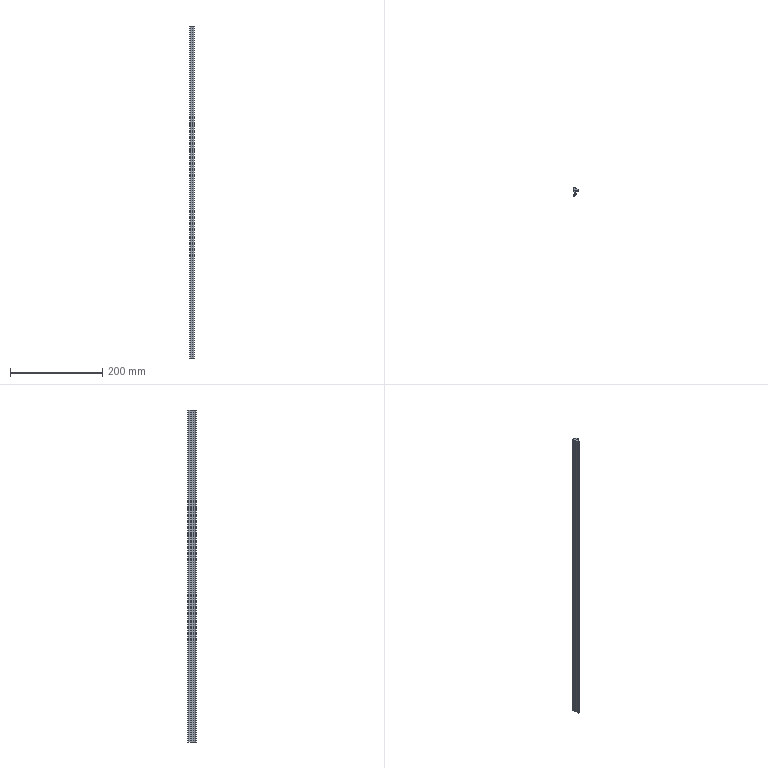Part | STEP file | AMH71封条-408 | 1 solid | 20 faces | box 10.8 x 17.5 x 720 mm | volume 56736 mm3 | cylinder 11 | plane 9 | commonest cylinder face diameters 1.6 x2 14 x2 0.4 x1 0.6 x1 0.8 x1 2.6 x1
STEP:
#1=CARTESIAN_POINT('',(-3.236,-11.055,0.));
#2=VERTEX_POINT('',#1);
#3=CARTESIAN_POINT('',(-4.3,-10.3,0.));
#4=VERTEX_POINT('',#3);
#5=CARTESIAN_POINT('',(-3.5,-10.3,0.));
#6=DIRECTION('',(0.,0.,-1.));
#7=DIRECTION('',(-1.,0.,0.));
#8=AXIS2_PLACEMENT_3D('',#5,#6,#7);
#9=CIRCLE('',#8,0.8);
#10=EDGE_CURVE('',#2,#4,#9,.T.);
#11=ORIENTED_EDGE('',*,*,#10,.T.);
#12=CARTESIAN_POINT('',(-4.3,-10.3,-720.));
#13=VERTEX_POINT('',#12);
#14=CARTESIAN_POINT('',(-4.3,-10.3,-100.));
#15=DIRECTION('',(0.,0.,-1.));
#16=VECTOR('',#15,1000.);
#17=LINE('',#14,#16);
#18=EDGE_CURVE('',#4,#13,#17,.T.);
#19=ORIENTED_EDGE('',*,*,#18,.T.);
#20=CARTESIAN_POINT('',(-3.236,-11.055,-720.));
#21=VERTEX_POINT('',#20);
#22=CARTESIAN_POINT('',(-3.5,-10.3,-720.));
#23=DIRECTION('',(0.,0.,1.));
#24=DIRECTION('',(-1.,0.,0.));
#25=AXIS2_PLACEMENT_3D('',#22,#23,#24);
#26=CIRCLE('',#25,0.8);
#27=EDGE_CURVE('',#13,#21,#26,.T.);
#28=ORIENTED_EDGE('',*,*,#27,.T.);
#29=CARTESIAN_POINT('',(-3.236,-11.055,-100.));
#30=DIRECTION('',(0.,0.,-1.));
#31=VECTOR('',#30,1000.);
#32=LINE('',#29,#31);
#33=EDGE_CURVE('',#2,#21,#32,.T.);
#34=ORIENTED_EDGE('',*,*,#33,.F.);
#35=EDGE_LOOP('',(#11,#19,#28,#34));
#36=FACE_OUTER_BOUND('',#35,.T.);
#37=CARTESIAN_POINT('',(-3.5,-10.3,-100.));
#38=DIRECTION('',(0.,0.,-1.));
#39=DIRECTION('',(-1.,0.,0.));
#40=AXIS2_PLACEMENT_3D('',#37,#38,#39);
#41=CYLINDRICAL_SURFACE('',#40,0.8);
#42=ADVANCED_FACE('',(#36),#41,.T.);
#43=CARTESIAN_POINT('',(1.184,-6.397,-720.));
#44=VERTEX_POINT('',#43);
#45=CARTESIAN_POINT('',(-5.702,-4.29,-720.));
#46=DIRECTION('',(0.,0.,1.));
#47=DIRECTION('',(-1.,0.,0.));
#48=AXIS2_PLACEMENT_3D('',#45,#46,#47);
#49=CIRCLE('',#48,7.201);
#50=EDGE_CURVE('',#21,#44,#49,.T.);
#51=ORIENTED_EDGE('',*,*,#50,.T.);
#52=CARTESIAN_POINT('',(1.184,-6.397,0.));
#53=VERTEX_POINT('',#52);
#54=CARTESIAN_POINT('',(1.184,-6.397,-100.));
#55=DIRECTION('',(0.,0.,1.));
#56=VECTOR('',#55,1000.);
#57=LINE('',#54,#56);
#58=EDGE_CURVE('',#44,#53,#57,.T.);
#59=ORIENTED_EDGE('',*,*,#58,.T.);
#60=CARTESIAN_POINT('',(-5.702,-4.29,0.));
#61=DIRECTION('',(0.,0.,-1.));
#62=DIRECTION('',(-1.,0.,0.));
#63=AXIS2_PLACEMENT_3D('',#60,#61,#62);
#64=CIRCLE('',#63,7.201);
#65=EDGE_CURVE('',#53,#2,#64,.T.);
#66=ORIENTED_EDGE('',*,*,#65,.T.);
#67=ORIENTED_EDGE('',*,*,#33,.T.);
#68=EDGE_LOOP('',(#51,#59,#66,#67));
#69=FACE_OUTER_BOUND('',#68,.T.);
#70=CARTESIAN_POINT('',(-5.702,-4.29,-100.));
#71=DIRECTION('',(0.,0.,-1.));
#72=DIRECTION('',(-1.,0.,0.));
#73=AXIS2_PLACEMENT_3D('',#70,#71,#72);
#74=CYLINDRICAL_SURFACE('',#73,7.201);
#75=ADVANCED_FACE('',(#69),#74,.T.);
#76=CARTESIAN_POINT('',(0.9,-6.,-720.));
#77=VERTEX_POINT('',#76);
#78=CARTESIAN_POINT('',(0.9,-6.3,-720.));
#79=DIRECTION('',(0.,0.,1.));
#80=DIRECTION('',(-1.,0.,0.));
#81=AXIS2_PLACEMENT_3D('',#78,#79,#80);
#82=CIRCLE('',#81,0.3);
#83=EDGE_CURVE('',#44,#77,#82,.T.);
#84=ORIENTED_EDGE('',*,*,#83,.T.);
#85=CARTESIAN_POINT('',(0.9,-6.,0.));
#86=VERTEX_POINT('',#85);
#87=CARTESIAN_POINT('',(0.9,-6.,-100.));
#88=DIRECTION('',(0.,0.,1.));
#89=VECTOR('',#88,1000.);
#90=LINE('',#87,#89);
#91=EDGE_CURVE('',#77,#86,#90,.T.);
#92=ORIENTED_EDGE('',*,*,#91,.T.);
#93=CARTESIAN_POINT('',(0.9,-6.3,0.));
#94=DIRECTION('',(0.,0.,-1.));
#95=DIRECTION('',(-1.,0.,0.));
#96=AXIS2_PLACEMENT_3D('',#93,#94,#95);
#97=CIRCLE('',#96,0.3);
#98=EDGE_CURVE('',#86,#53,#97,.T.);
#99=ORIENTED_EDGE('',*,*,#98,.T.);
#100=ORIENTED_EDGE('',*,*,#58,.F.);
#101=EDGE_LOOP('',(#84,#92,#99,#100));
#102=FACE_OUTER_BOUND('',#101,.T.);
#103=CARTESIAN_POINT('',(0.9,-6.3,-100.));
#104=DIRECTION('',(0.,0.,-1.));
#105=DIRECTION('',(-1.,0.,0.));
#106=AXIS2_PLACEMENT_3D('',#103,#104,#105);
#107=CYLINDRICAL_SURFACE('',#106,0.3);
#108=ADVANCED_FACE('',(#102),#107,.T.);
#109=CARTESIAN_POINT('',(-2.5,-0.5,-720.));
#110=VERTEX_POINT('',#109);
#111=CARTESIAN_POINT('',(-2.5,-6.153,-720.));
#112=VERTEX_POINT('',#111);
#113=CARTESIAN_POINT('',(-2.5,-6.397,-720.));
#114=DIRECTION('',(0.,-1.,0.));
#115=VECTOR('',#114,1000.);
#116=LINE('',#113,#115);
#117=EDGE_CURVE('',#110,#112,#116,.T.);
#118=ORIENTED_EDGE('',*,*,#117,.F.);
#119=CARTESIAN_POINT('',(-4.2,1.695,-720.));
#120=VERTEX_POINT('',#119);
#121=CARTESIAN_POINT('',(-1.701,1.875,-720.));
#122=DIRECTION('',(0.,0.,1.));
#123=DIRECTION('',(-1.,0.,0.));
#124=AXIS2_PLACEMENT_3D('',#121,#122,#123);
#125=CIRCLE('',#124,2.506);
#126=EDGE_CURVE('',#120,#110,#125,.T.);
#127=ORIENTED_EDGE('',*,*,#126,.F.);
#128=CARTESIAN_POINT('',(-4.2,5.1,-720.));
#129=VERTEX_POINT('',#128);
#130=CARTESIAN_POINT('',(-4.2,-6.397,-720.));
#131=DIRECTION('',(0.,-1.,0.));
#132=VECTOR('',#131,1000.);
#133=LINE('',#130,#132);
#134=EDGE_CURVE('',#129,#120,#133,.T.);
#135=ORIENTED_EDGE('',*,*,#134,.F.);
#136=CARTESIAN_POINT('',(-2.892,6.4,-720.));
#137=VERTEX_POINT('',#136);
#138=CARTESIAN_POINT('',(-2.9,5.1,-720.));
#139=DIRECTION('',(0.,0.,1.));
#140=DIRECTION('',(-1.,0.,0.));
#141=AXIS2_PLACEMENT_3D('',#138,#139,#140);
#142=CIRCLE('',#141,1.3);
#143=EDGE_CURVE('',#137,#129,#142,.T.);
#144=ORIENTED_EDGE('',*,*,#143,.F.);
#145=CARTESIAN_POINT('',(0.5,5.5,-720.));
#146=VERTEX_POINT('',#145);
#147=CARTESIAN_POINT('',(-2.934,-0.5999,-720.));
#148=DIRECTION('',(0.,0.,1.));
#149=DIRECTION('',(-1.,0.,0.));
#150=AXIS2_PLACEMENT_3D('',#147,#148,#149);
#151=CIRCLE('',#150,7.);
#152=EDGE_CURVE('',#146,#137,#151,.T.);
#153=ORIENTED_EDGE('',*,*,#152,.F.);
#154=CARTESIAN_POINT('',(5.5,1.7,-720.));
#155=VERTEX_POINT('',#154);
#156=CARTESIAN_POINT('',(5.5,1.7,-720.));
#157=DIRECTION('',(-0.7962,0.6051,0.));
#158=VECTOR('',#157,1000.);
#159=LINE('',#156,#158);
#160=EDGE_CURVE('',#155,#146,#159,.T.);
#161=ORIENTED_EDGE('',*,*,#160,.F.);
#162=CARTESIAN_POINT('',(6.458,-0.2215,-720.));
#163=VERTEX_POINT('',#162);
#164=CARTESIAN_POINT('',(6.458,-0.2215,-720.));
#165=DIRECTION('',(-0.4462,0.8949,0.));
#166=VECTOR('',#165,1000.);
#167=LINE('',#164,#166);
#168=EDGE_CURVE('',#163,#155,#167,.T.);
#169=ORIENTED_EDGE('',*,*,#168,.F.);
#170=CARTESIAN_POINT('',(5.895,-0.7433,-720.));
#171=VERTEX_POINT('',#170);
#172=CARTESIAN_POINT('',(6.1,-0.4,-720.));
#173=DIRECTION('',(0.,0.,1.));
#174=DIRECTION('',(-1.,0.,0.));
#175=AXIS2_PLACEMENT_3D('',#172,#173,#174);
#176=CIRCLE('',#175,0.4);
#177=EDGE_CURVE('',#171,#163,#176,.T.);
#178=ORIENTED_EDGE('',*,*,#177,.F.);
#179=CARTESIAN_POINT('',(3.,0.,-720.));
#180=VERTEX_POINT('',#179);
#181=CARTESIAN_POINT('',(2.746,-6.995,-720.));
#182=DIRECTION('',(0.,0.,-1.));
#183=DIRECTION('',(-1.,0.,0.));
#184=AXIS2_PLACEMENT_3D('',#181,#182,#183);
#185=CIRCLE('',#184,7.);
#186=EDGE_CURVE('',#180,#171,#185,.T.);
#187=ORIENTED_EDGE('',*,*,#186,.F.);
#188=CARTESIAN_POINT('',(0.,0.,-720.));
#189=VERTEX_POINT('',#188);
#190=CARTESIAN_POINT('',(-6.814,0.,-720.));
#191=DIRECTION('',(1.,0.,0.));
#192=VECTOR('',#191,1000.);
#193=LINE('',#190,#192);
#194=EDGE_CURVE('',#189,#180,#193,.T.);
#195=ORIENTED_EDGE('',*,*,#194,.F.);
#196=CARTESIAN_POINT('',(0.,-5.8,-720.));
#197=VERTEX_POINT('',#196);
#198=CARTESIAN_POINT('',(0.,-6.397,-720.));
#199=DIRECTION('',(0.,1.,0.));
#200=VECTOR('',#199,1000.);
#201=LINE('',#198,#200);
#202=EDGE_CURVE('',#197,#189,#201,.T.);
#203=ORIENTED_EDGE('',*,*,#202,.F.);
#204=CARTESIAN_POINT('',(0.2,-6.,-720.));
#205=VERTEX_POINT('',#204);
#206=CARTESIAN_POINT('',(0.2,-5.8,-720.));
#207=DIRECTION('',(0.,0.,1.));
#208=DIRECTION('',(-1.,0.,0.));
#209=AXIS2_PLACEMENT_3D('',#206,#207,#208);
#210=CIRCLE('',#209,0.2);
#211=EDGE_CURVE('',#197,#205,#210,.T.);
#212=ORIENTED_EDGE('',*,*,#211,.T.);
#213=CARTESIAN_POINT('',(-6.814,-6.,-720.));
#214=DIRECTION('',(-1.,0.,0.));
#215=VECTOR('',#214,1000.);
#216=LINE('',#213,#215);
#217=EDGE_CURVE('',#77,#205,#216,.T.);
#218=ORIENTED_EDGE('',*,*,#217,.F.);
#219=ORIENTED_EDGE('',*,*,#83,.F.);
#220=ORIENTED_EDGE('',*,*,#50,.F.);
#221=ORIENTED_EDGE('',*,*,#27,.F.);
#222=CARTESIAN_POINT('',(-3.998,-9.674,-720.));
#223=VERTEX_POINT('',#222);
#224=CARTESIAN_POINT('',(-3.5,-10.3,-720.));
#225=DIRECTION('',(0.,0.,1.));
#226=DIRECTION('',(-1.,0.,0.));
#227=AXIS2_PLACEMENT_3D('',#224,#225,#226);
#228=CIRCLE('',#227,0.8);
#229=EDGE_CURVE('',#223,#13,#228,.T.);
#230=ORIENTED_EDGE('',*,*,#229,.F.);
#231=CARTESIAN_POINT('',(-6.814,-6.397,-720.));
#232=DIRECTION('',(0.,0.,-1.));
#233=DIRECTION('',(-1.,0.,0.));
#234=AXIS2_PLACEMENT_3D('',#231,#232,#233);
#235=CIRCLE('',#234,4.321);
#236=EDGE_CURVE('',#112,#223,#235,.T.);
#237=ORIENTED_EDGE('',*,*,#236,.F.);
#238=EDGE_LOOP('',(#118,#127,#135,#144,#153,#161,#169,#178,#187,#195,#203,#212,#218,#219,#220,#221,#230,#237));
#239=FACE_OUTER_BOUND('',#238,.T.);
#240=CARTESIAN_POINT('',(-6.814,-6.397,-720.));
#241=DIRECTION('',(0.,0.,1.));
#242=DIRECTION('',(1.,0.,0.));
#243=AXIS2_PLACEMENT_3D('',#240,#241,#242);
#244=PLANE('',#243);
#245=ADVANCED_FACE('',(#239),#244,.F.);
#246=ORIENTED_EDGE('',*,*,#18,.F.);
#247=CARTESIAN_POINT('',(-3.998,-9.674,0.));
#248=VERTEX_POINT('',#247);
#249=CARTESIAN_POINT('',(-3.5,-10.3,0.));
#250=DIRECTION('',(0.,0.,-1.));
#251=DIRECTION('',(-1.,0.,0.));
#252=AXIS2_PLACEMENT_3D('',#249,#250,#251);
#253=CIRCLE('',#252,0.8);
#254=EDGE_CURVE('',#4,#248,#253,.T.);
#255=ORIENTED_EDGE('',*,*,#254,.T.);
#256=CARTESIAN_POINT('',(-3.998,-9.674,-100.));
#257=DIRECTION('',(0.,0.,-1.));
#258=VECTOR('',#257,1000.);
#259=LINE('',#256,#258);
#260=EDGE_CURVE('',#248,#223,#259,.T.);
#261=ORIENTED_EDGE('',*,*,#260,.T.);
#262=ORIENTED_EDGE('',*,*,#229,.T.);
#263=EDGE_LOOP('',(#246,#255,#261,#262));
#264=FACE_OUTER_BOUND('',#263,.T.);
#265=CARTESIAN_POINT('',(-3.5,-10.3,-100.));
#266=DIRECTION('',(0.,0.,-1.));
#267=DIRECTION('',(-1.,0.,0.));
#268=AXIS2_PLACEMENT_3D('',#265,#266,#267);
#269=CYLINDRICAL_SURFACE('',#268,0.8);
#270=ADVANCED_FACE('',(#264),#269,.T.);
#271=CARTESIAN_POINT('',(-4.2,1.695,0.));
#272=VERTEX_POINT('',#271);
#273=CARTESIAN_POINT('',(-2.5,-0.5,0.));
#274=VERTEX_POINT('',#273);
#275=CARTESIAN_POINT('',(-1.701,1.875,0.));
#276=DIRECTION('',(0.,0.,1.));
#277=DIRECTION('',(-1.,0.,0.));
#278=AXIS2_PLACEMENT_3D('',#275,#276,#277);
#279=CIRCLE('',#278,2.506);
#280=EDGE_CURVE('',#272,#274,#279,.T.);
#281=ORIENTED_EDGE('',*,*,#280,.T.);
#282=CARTESIAN_POINT('',(-2.5,-6.153,0.));
#283=VERTEX_POINT('',#282);
#284=CARTESIAN_POINT('',(-2.5,-6.397,0.));
#285=DIRECTION('',(0.,-1.,0.));
#286=VECTOR('',#285,1000.);
#287=LINE('',#284,#286);
#288=EDGE_CURVE('',#274,#283,#287,.T.);
#289=ORIENTED_EDGE('',*,*,#288,.T.);
#290=CARTESIAN_POINT('',(-6.814,-6.397,0.));
#291=DIRECTION('',(0.,0.,-1.));
#292=DIRECTION('',(-1.,0.,0.));
#293=AXIS2_PLACEMENT_3D('',#290,#291,#292);
#294=CIRCLE('',#293,4.321);
#295=EDGE_CURVE('',#283,#248,#294,.T.);
#296=ORIENTED_EDGE('',*,*,#295,.T.);
#297=ORIENTED_EDGE('',*,*,#254,.F.);
#298=ORIENTED_EDGE('',*,*,#10,.F.);
#299=ORIENTED_EDGE('',*,*,#65,.F.);
#300=ORIENTED_EDGE('',*,*,#98,.F.);
#301=CARTESIAN_POINT('',(0.2,-6.,0.));
#302=VERTEX_POINT('',#301);
#303=CARTESIAN_POINT('',(-6.814,-6.,0.));
#304=DIRECTION('',(-1.,0.,0.));
#305=VECTOR('',#304,1000.);
#306=LINE('',#303,#305);
#307=EDGE_CURVE('',#86,#302,#306,.T.);
#308=ORIENTED_EDGE('',*,*,#307,.T.);
#309=CARTESIAN_POINT('',(0.,-5.8,0.));
#310=VERTEX_POINT('',#309);
#311=CARTESIAN_POINT('',(0.2,-5.8,0.));
#312=DIRECTION('',(0.,0.,-1.));
#313=DIRECTION('',(-1.,0.,0.));
#314=AXIS2_PLACEMENT_3D('',#311,#312,#313);
#315=CIRCLE('',#314,0.2);
#316=EDGE_CURVE('',#302,#310,#315,.T.);
#317=ORIENTED_EDGE('',*,*,#316,.T.);
#318=CARTESIAN_POINT('',(0.,0.,0.));
#319=VERTEX_POINT('',#318);
#320=CARTESIAN_POINT('',(0.,-6.397,0.));
#321=DIRECTION('',(0.,1.,0.));
#322=VECTOR('',#321,1000.);
#323=LINE('',#320,#322);
#324=EDGE_CURVE('',#310,#319,#323,.T.);
#325=ORIENTED_EDGE('',*,*,#324,.T.);
#326=CARTESIAN_POINT('',(3.,0.,0.));
#327=VERTEX_POINT('',#326);
#328=CARTESIAN_POINT('',(-6.814,0.,0.));
#329=DIRECTION('',(1.,0.,0.));
#330=VECTOR('',#329,1000.);
#331=LINE('',#328,#330);
#332=EDGE_CURVE('',#319,#327,#331,.T.);
#333=ORIENTED_EDGE('',*,*,#332,.T.);
#334=CARTESIAN_POINT('',(5.895,-0.7433,0.));
#335=VERTEX_POINT('',#334);
#336=CARTESIAN_POINT('',(2.746,-6.995,0.));
#337=DIRECTION('',(0.,0.,-1.));
#338=DIRECTION('',(-1.,0.,0.));
#339=AXIS2_PLACEMENT_3D('',#336,#337,#338);
#340=CIRCLE('',#339,7.);
#341=EDGE_CURVE('',#327,#335,#340,.T.);
#342=ORIENTED_EDGE('',*,*,#341,.T.);
#343=CARTESIAN_POINT('',(6.458,-0.2215,0.));
#344=VERTEX_POINT('',#343);
#345=CARTESIAN_POINT('',(6.1,-0.4,0.));
#346=DIRECTION('',(0.,0.,-1.));
#347=DIRECTION('',(-1.,0.,0.));
#348=AXIS2_PLACEMENT_3D('',#345,#346,#347);
#349=CIRCLE('',#348,0.4);
#350=EDGE_CURVE('',#344,#335,#349,.T.);
#351=ORIENTED_EDGE('',*,*,#350,.F.);
#352=CARTESIAN_POINT('',(5.5,1.7,0.));
#353=VERTEX_POINT('',#352);
#354=CARTESIAN_POINT('',(6.458,-0.2215,0.));
#355=DIRECTION('',(-0.4462,0.8949,0.));
#356=VECTOR('',#355,1000.);
#357=LINE('',#354,#356);
#358=EDGE_CURVE('',#344,#353,#357,.T.);
#359=ORIENTED_EDGE('',*,*,#358,.T.);
#360=CARTESIAN_POINT('',(0.5,5.5,0.));
#361=VERTEX_POINT('',#360);
#362=CARTESIAN_POINT('',(5.5,1.7,0.));
#363=DIRECTION('',(-0.7962,0.6051,0.));
#364=VECTOR('',#363,1000.);
#365=LINE('',#362,#364);
#366=EDGE_CURVE('',#353,#361,#365,.T.);
#367=ORIENTED_EDGE('',*,*,#366,.T.);
#368=CARTESIAN_POINT('',(-2.892,6.4,0.));
#369=VERTEX_POINT('',#368);
#370=CARTESIAN_POINT('',(-2.934,-0.5999,0.));
#371=DIRECTION('',(0.,0.,1.));
#372=DIRECTION('',(-1.,0.,0.));
#373=AXIS2_PLACEMENT_3D('',#370,#371,#372);
#374=CIRCLE('',#373,7.);
#375=EDGE_CURVE('',#361,#369,#374,.T.);
#376=ORIENTED_EDGE('',*,*,#375,.T.);
#377=CARTESIAN_POINT('',(-4.2,5.1,0.));
#378=VERTEX_POINT('',#377);
#379=CARTESIAN_POINT('',(-2.9,5.1,0.));
#380=DIRECTION('',(0.,0.,1.));
#381=DIRECTION('',(-1.,0.,0.));
#382=AXIS2_PLACEMENT_3D('',#379,#380,#381);
#383=CIRCLE('',#382,1.3);
#384=EDGE_CURVE('',#369,#378,#383,.T.);
#385=ORIENTED_EDGE('',*,*,#384,.T.);
#386=CARTESIAN_POINT('',(-4.2,-6.397,0.));
#387=DIRECTION('',(0.,-1.,0.));
#388=VECTOR('',#387,1000.);
#389=LINE('',#386,#388);
#390=EDGE_CURVE('',#378,#272,#389,.T.);
#391=ORIENTED_EDGE('',*,*,#390,.T.);
#392=EDGE_LOOP('',(#281,#289,#296,#297,#298,#299,#300,#308,#317,#325,#333,#342,#351,#359,#367,#376,#385,#391));
#393=FACE_OUTER_BOUND('',#392,.T.);
#394=CARTESIAN_POINT('',(-6.814,-6.397,0.));
#395=DIRECTION('',(0.,0.,1.));
#396=DIRECTION('',(1.,0.,0.));
#397=AXIS2_PLACEMENT_3D('',#394,#395,#396);
#398=PLANE('',#397);
#399=ADVANCED_FACE('',(#393),#398,.T.);
#400=ORIENTED_EDGE('',*,*,#217,.T.);
#401=CARTESIAN_POINT('',(0.2,-6.,-100.));
#402=DIRECTION('',(0.,0.,1.));
#403=VECTOR('',#402,1000.);
#404=LINE('',#401,#403);
#405=EDGE_CURVE('',#205,#302,#404,.T.);
#406=ORIENTED_EDGE('',*,*,#405,.T.);
#407=ORIENTED_EDGE('',*,*,#307,.F.);
#408=ORIENTED_EDGE('',*,*,#91,.F.);
#409=EDGE_LOOP('',(#400,#406,#407,#408));
#410=FACE_OUTER_BOUND('',#409,.T.);
#411=CARTESIAN_POINT('',(0.9,-6.,-100.));
#412=DIRECTION('',(0.,1.,0.));
#413=DIRECTION('',(0.,0.,1.));
#414=AXIS2_PLACEMENT_3D('',#411,#412,#413);
#415=PLANE('',#414);
#416=ADVANCED_FACE('',(#410),#415,.T.);
#417=CARTESIAN_POINT('',(-2.5,-6.153,-100.));
#418=DIRECTION('',(0.,0.,1.));
#419=VECTOR('',#418,1000.);
#420=LINE('',#417,#419);
#421=EDGE_CURVE('',#112,#283,#420,.T.);
#422=ORIENTED_EDGE('',*,*,#421,.F.);
#423=ORIENTED_EDGE('',*,*,#236,.T.);
#424=ORIENTED_EDGE('',*,*,#260,.F.);
#425=ORIENTED_EDGE('',*,*,#295,.F.);
#426=EDGE_LOOP('',(#422,#423,#424,#425));
#427=FACE_OUTER_BOUND('',#426,.T.);
#428=CARTESIAN_POINT('',(-6.814,-6.397,-100.));
#429=DIRECTION('',(0.,0.,-1.));
#430=DIRECTION('',(-1.,0.,0.));
#431=AXIS2_PLACEMENT_3D('',#428,#429,#430);
#432=CYLINDRICAL_SURFACE('',#431,4.321);
#433=ADVANCED_FACE('',(#427),#432,.F.);
#434=ORIENTED_EDGE('',*,*,#117,.T.);
#435=ORIENTED_EDGE('',*,*,#421,.T.);
#436=ORIENTED_EDGE('',*,*,#288,.F.);
#437=CARTESIAN_POINT('',(-2.5,-0.5,-100.));
#438=DIRECTION('',(0.,0.,-1.));
#439=VECTOR('',#438,1000.);
#440=LINE('',#437,#439);
#441=EDGE_CURVE('',#274,#110,#440,.T.);
#442=ORIENTED_EDGE('',*,*,#441,.T.);
#443=EDGE_LOOP('',(#434,#435,#436,#442));
#444=FACE_OUTER_BOUND('',#443,.T.);
#445=CARTESIAN_POINT('',(-2.5,-0.5,-100.));
#446=DIRECTION('',(-1.,0.,0.));
#447=DIRECTION('',(0.,0.,1.));
#448=AXIS2_PLACEMENT_3D('',#445,#446,#447);
#449=PLANE('',#448);
#450=ADVANCED_FACE('',(#444),#449,.T.);
#451=ORIENTED_EDGE('',*,*,#126,.T.);
#452=ORIENTED_EDGE('',*,*,#441,.F.);
#453=ORIENTED_EDGE('',*,*,#280,.F.);
#454=CARTESIAN_POINT('',(-4.2,1.695,-100.));
#455=DIRECTION('',(0.,0.,-1.));
#456=VECTOR('',#455,1000.);
#457=LINE('',#454,#456);
#458=EDGE_CURVE('',#272,#120,#457,.T.);
#459=ORIENTED_EDGE('',*,*,#458,.T.);
#460=EDGE_LOOP('',(#451,#452,#453,#459));
#461=FACE_OUTER_BOUND('',#460,.T.);
#462=CARTESIAN_POINT('',(-1.701,1.875,-100.));
#463=DIRECTION('',(0.,0.,-1.));
#464=DIRECTION('',(-1.,0.,0.));
#465=AXIS2_PLACEMENT_3D('',#462,#463,#464);
#466=CYLINDRICAL_SURFACE('',#465,2.506);
#467=ADVANCED_FACE('',(#461),#466,.T.);
#468=ORIENTED_EDGE('',*,*,#134,.T.);
#469=ORIENTED_EDGE('',*,*,#458,.F.);
#470=ORIENTED_EDGE('',*,*,#390,.F.);
#471=CARTESIAN_POINT('',(-4.2,5.1,-100.));
#472=DIRECTION('',(0.,0.,-1.));
#473=VECTOR('',#472,1000.);
#474=LINE('',#471,#473);
#475=EDGE_CURVE('',#378,#129,#474,.T.);
#476=ORIENTED_EDGE('',*,*,#475,.T.);
#477=EDGE_LOOP('',(#468,#469,#470,#476));
#478=FACE_OUTER_BOUND('',#477,.T.);
#479=CARTESIAN_POINT('',(-4.2,5.1,-100.));
#480=DIRECTION('',(-1.,0.,0.));
#481=DIRECTION('',(0.,0.,1.));
#482=AXIS2_PLACEMENT_3D('',#479,#480,#481);
#483=PLANE('',#482);
#484=ADVANCED_FACE('',(#478),#483,.T.);
#485=ORIENTED_EDGE('',*,*,#143,.T.);
#486=ORIENTED_EDGE('',*,*,#475,.F.);
#487=ORIENTED_EDGE('',*,*,#384,.F.);
#488=CARTESIAN_POINT('',(-2.892,6.4,-100.));
#489=DIRECTION('',(0.,0.,-1.));
#490=VECTOR('',#489,1000.);
#491=LINE('',#488,#490);
#492=EDGE_CURVE('',#369,#137,#491,.T.);
#493=ORIENTED_EDGE('',*,*,#492,.T.);
#494=EDGE_LOOP('',(#485,#486,#487,#493));
#495=FACE_OUTER_BOUND('',#494,.T.);
#496=CARTESIAN_POINT('',(-2.9,5.1,-100.));
#497=DIRECTION('',(0.,0.,-1.));
#498=DIRECTION('',(-1.,0.,0.));
#499=AXIS2_PLACEMENT_3D('',#496,#497,#498);
#500=CYLINDRICAL_SURFACE('',#499,1.3);
#501=ADVANCED_FACE('',(#495),#500,.T.);
#502=ORIENTED_EDGE('',*,*,#152,.T.);
#503=ORIENTED_EDGE('',*,*,#492,.F.);
#504=ORIENTED_EDGE('',*,*,#375,.F.);
#505=CARTESIAN_POINT('',(0.5,5.5,-100.));
#506=DIRECTION('',(0.,0.,-1.));
#507=VECTOR('',#506,1000.);
#508=LINE('',#505,#507);
#509=EDGE_CURVE('',#361,#146,#508,.T.);
#510=ORIENTED_EDGE('',*,*,#509,.T.);
#511=EDGE_LOOP('',(#502,#503,#504,#510));
#512=FACE_OUTER_BOUND('',#511,.T.);
#513=CARTESIAN_POINT('',(-2.934,-0.5999,-100.));
#514=DIRECTION('',(0.,0.,-1.));
#515=DIRECTION('',(-1.,0.,0.));
#516=AXIS2_PLACEMENT_3D('',#513,#514,#515);
#517=CYLINDRICAL_SURFACE('',#516,7.);
#518=ADVANCED_FACE('',(#512),#517,.T.);
#519=ORIENTED_EDGE('',*,*,#160,.T.);
#520=ORIENTED_EDGE('',*,*,#509,.F.);
#521=ORIENTED_EDGE('',*,*,#366,.F.);
#522=CARTESIAN_POINT('',(5.5,1.7,-100.));
#523=DIRECTION('',(0.,0.,-1.));
#524=VECTOR('',#523,1000.);
#525=LINE('',#522,#524);
#526=EDGE_CURVE('',#353,#155,#525,.T.);
#527=ORIENTED_EDGE('',*,*,#526,.T.);
#528=EDGE_LOOP('',(#519,#520,#521,#527));
#529=FACE_OUTER_BOUND('',#528,.T.);
#530=CARTESIAN_POINT('',(5.5,1.7,-100.));
#531=DIRECTION('',(0.6051,0.7962,0.));
#532=DIRECTION('',(-0.7962,0.6051,0.));
#533=AXIS2_PLACEMENT_3D('',#530,#531,#532);
#534=PLANE('',#533);
#535=ADVANCED_FACE('',(#529),#534,.T.);
#536=ORIENTED_EDGE('',*,*,#168,.T.);
#537=ORIENTED_EDGE('',*,*,#526,.F.);
#538=ORIENTED_EDGE('',*,*,#358,.F.);
#539=CARTESIAN_POINT('',(6.458,-0.2215,-100.));
#540=DIRECTION('',(0.,0.,-1.));
#541=VECTOR('',#540,1000.);
#542=LINE('',#539,#541);
#543=EDGE_CURVE('',#344,#163,#542,.T.);
#544=ORIENTED_EDGE('',*,*,#543,.T.);
#545=EDGE_LOOP('',(#536,#537,#538,#544));
#546=FACE_OUTER_BOUND('',#545,.T.);
#547=CARTESIAN_POINT('',(6.458,-0.2215,-100.));
#548=DIRECTION('',(0.8949,0.4462,0.));
#549=DIRECTION('',(-0.4462,0.8949,0.));
#550=AXIS2_PLACEMENT_3D('',#547,#548,#549);
#551=PLANE('',#550);
#552=ADVANCED_FACE('',(#546),#551,.T.);
#553=CARTESIAN_POINT('',(3.,0.,-100.));
#554=DIRECTION('',(0.,0.,1.));
#555=VECTOR('',#554,1000.);
#556=LINE('',#553,#555);
#557=EDGE_CURVE('',#180,#327,#556,.T.);
#558=ORIENTED_EDGE('',*,*,#557,.F.);
#559=ORIENTED_EDGE('',*,*,#186,.T.);
#560=CARTESIAN_POINT('',(5.895,-0.7433,-100.));
#561=DIRECTION('',(0.,0.,-1.));
#562=VECTOR('',#561,1000.);
#563=LINE('',#560,#562);
#564=EDGE_CURVE('',#335,#171,#563,.T.);
#565=ORIENTED_EDGE('',*,*,#564,.F.);
#566=ORIENTED_EDGE('',*,*,#341,.F.);
#567=EDGE_LOOP('',(#558,#559,#565,#566));
#568=FACE_OUTER_BOUND('',#567,.T.);
#569=CARTESIAN_POINT('',(2.746,-6.995,-100.));
#570=DIRECTION('',(0.,0.,-1.));
#571=DIRECTION('',(-1.,0.,0.));
#572=AXIS2_PLACEMENT_3D('',#569,#570,#571);
#573=CYLINDRICAL_SURFACE('',#572,7.);
#574=ADVANCED_FACE('',(#568),#573,.F.);
#575=ORIENTED_EDGE('',*,*,#194,.T.);
#576=ORIENTED_EDGE('',*,*,#557,.T.);
#577=ORIENTED_EDGE('',*,*,#332,.F.);
#578=CARTESIAN_POINT('',(0.,0.,-100.));
#579=DIRECTION('',(0.,0.,-1.));
#580=VECTOR('',#579,1000.);
#581=LINE('',#578,#580);
#582=EDGE_CURVE('',#319,#189,#581,.T.);
#583=ORIENTED_EDGE('',*,*,#582,.T.);
#584=EDGE_LOOP('',(#575,#576,#577,#583));
#585=FACE_OUTER_BOUND('',#584,.T.);
#586=CARTESIAN_POINT('',(0.,0.,-100.));
#587=DIRECTION('',(0.,-1.,0.));
#588=DIRECTION('',(0.,0.,-1.));
#589=AXIS2_PLACEMENT_3D('',#586,#587,#588);
#590=PLANE('',#589);
#591=ADVANCED_FACE('',(#585),#590,.T.);
#592=ORIENTED_EDGE('',*,*,#202,.T.);
#593=ORIENTED_EDGE('',*,*,#582,.F.);
#594=ORIENTED_EDGE('',*,*,#324,.F.);
#595=CARTESIAN_POINT('',(0.,-5.8,-100.));
#596=DIRECTION('',(0.,0.,-1.));
#597=VECTOR('',#596,1000.);
#598=LINE('',#595,#597);
#599=EDGE_CURVE('',#310,#197,#598,.T.);
#600=ORIENTED_EDGE('',*,*,#599,.T.);
#601=EDGE_LOOP('',(#592,#593,#594,#600));
#602=FACE_OUTER_BOUND('',#601,.T.);
#603=CARTESIAN_POINT('',(0.,-5.8,-100.));
#604=DIRECTION('',(1.,0.,0.));
#605=DIRECTION('',(0.,0.,-1.));
#606=AXIS2_PLACEMENT_3D('',#603,#604,#605);
#607=PLANE('',#606);
#608=ADVANCED_FACE('',(#602),#607,.T.);
#609=ORIENTED_EDGE('',*,*,#405,.F.);
#610=ORIENTED_EDGE('',*,*,#211,.F.);
#611=ORIENTED_EDGE('',*,*,#599,.F.);
#612=ORIENTED_EDGE('',*,*,#316,.F.);
#613=EDGE_LOOP('',(#609,#610,#611,#612));
#614=FACE_OUTER_BOUND('',#613,.T.);
#615=CARTESIAN_POINT('',(0.2,-5.8,-100.));
#616=DIRECTION('',(0.,0.,-1.));
#617=DIRECTION('',(-1.,0.,0.));
#618=AXIS2_PLACEMENT_3D('',#615,#616,#617);
#619=CYLINDRICAL_SURFACE('',#618,0.2);
#620=ADVANCED_FACE('',(#614),#619,.F.);
#621=ORIENTED_EDGE('',*,*,#177,.T.);
#622=ORIENTED_EDGE('',*,*,#543,.F.);
#623=ORIENTED_EDGE('',*,*,#350,.T.);
#624=ORIENTED_EDGE('',*,*,#564,.T.);
#625=EDGE_LOOP('',(#621,#622,#623,#624));
#626=FACE_OUTER_BOUND('',#625,.T.);
#627=CARTESIAN_POINT('',(6.1,-0.4,-100.));
#628=DIRECTION('',(0.,0.,-1.));
#629=DIRECTION('',(-1.,0.,0.));
#630=AXIS2_PLACEMENT_3D('',#627,#628,#629);
#631=CYLINDRICAL_SURFACE('',#630,0.4);
#632=ADVANCED_FACE('',(#626),#631,.T.);
#633=CLOSED_SHELL('',(#42,#75,#108,#245,#270,#399,#416,#433,#450,#467,#484,#501,#518,#535,#552,#574,#591,#608,#620,#632));
#634=MANIFOLD_SOLID_BREP('',#633);
#635=CARTESIAN_POINT('',(0.,0.,0.));
#636=DIRECTION('',(0.,0.,1.));
#637=DIRECTION('',(1.,0.,0.));
#638=AXIS2_PLACEMENT_3D('',#635,#636,#637);
#639=(LENGTH_UNIT()NAMED_UNIT(*)SI_UNIT(.MILLI.,.METRE.));
#640=UNCERTAINTY_MEASURE_WITH_UNIT(LENGTH_MEASURE(0.00001),#639,'','');
#641=(NAMED_UNIT(*)PLANE_ANGLE_UNIT()SI_UNIT($,.RADIAN.));
#642=(NAMED_UNIT(*)SI_UNIT($,.STERADIAN.)SOLID_ANGLE_UNIT());
#643=(GEOMETRIC_REPRESENTATION_CONTEXT(3)GLOBAL_UNCERTAINTY_ASSIGNED_CONTEXT((#640))GLOBAL_UNIT_ASSIGNED_CONTEXT((#639,#641,#642))REPRESENTATION_CONTEXT('',''));
#644=ADVANCED_BREP_SHAPE_REPRESENTATION('',(#634,#638),#643);